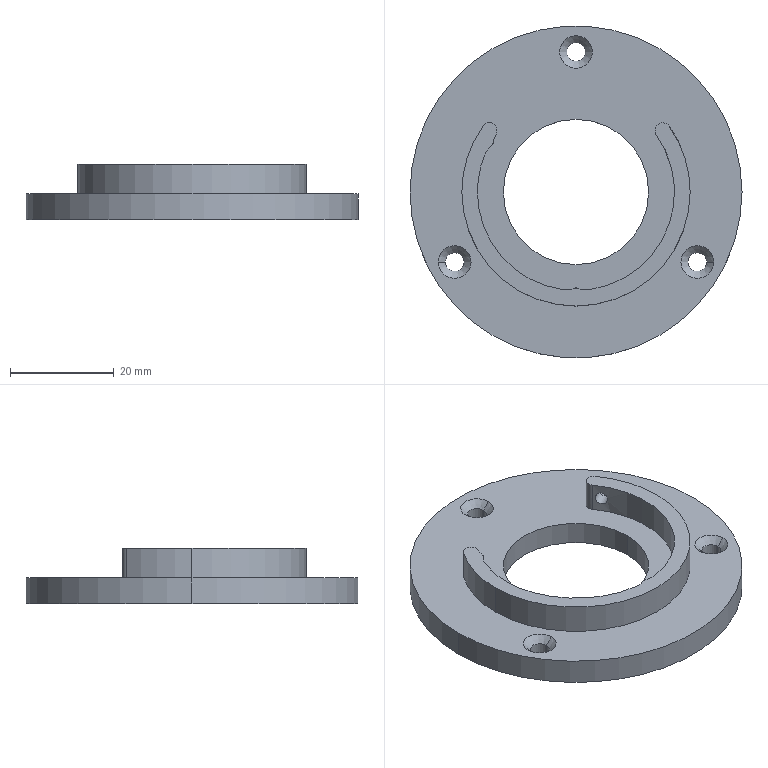Part | SolidWorks | features Fillet 3, ICE 3, HoleWzd 2, Extrusion 1 | 1 solid | 40 faces | box 64 x 64 x 10.7 mm | volume 13896 mm3 | cylinder 25 | cone 8 | plane 4 | spline 3 | commonest cylinder face diameters 3.6 x6 10 x3 38 x3 44 x3 2.5 x2 28 x2